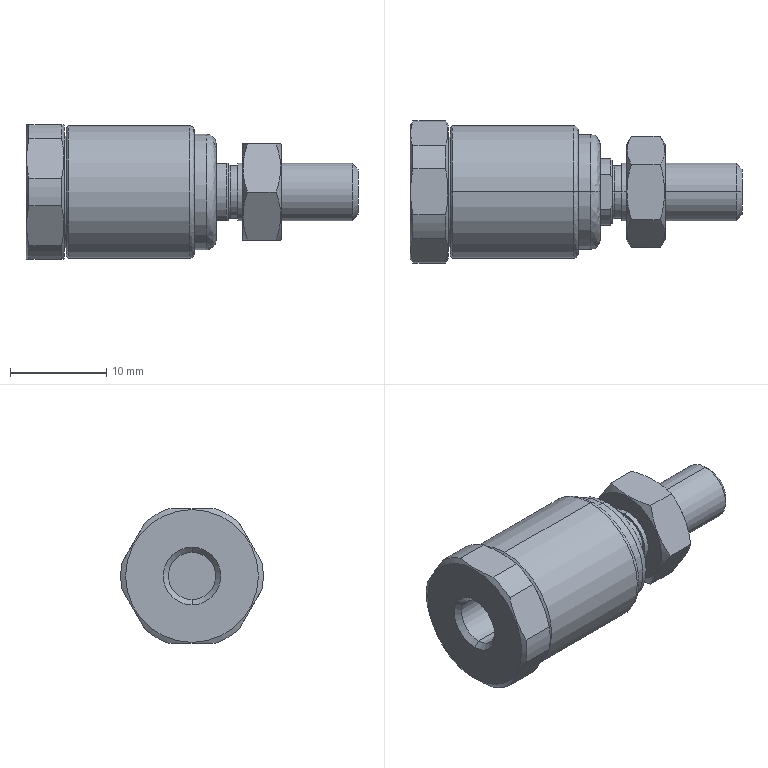Part | STEP file | F-M06100F | 1 solid | 75 faces | box 34.5 x 14.8 x 14 mm | volume 3405 mm3 | plane 27 | cylinder 22 | cone 18 | spline 8 | commonest cylinder face diameters 14.8 x6 6 x4 4.917 x2 5.5 x2 7 x2 11.6 x2